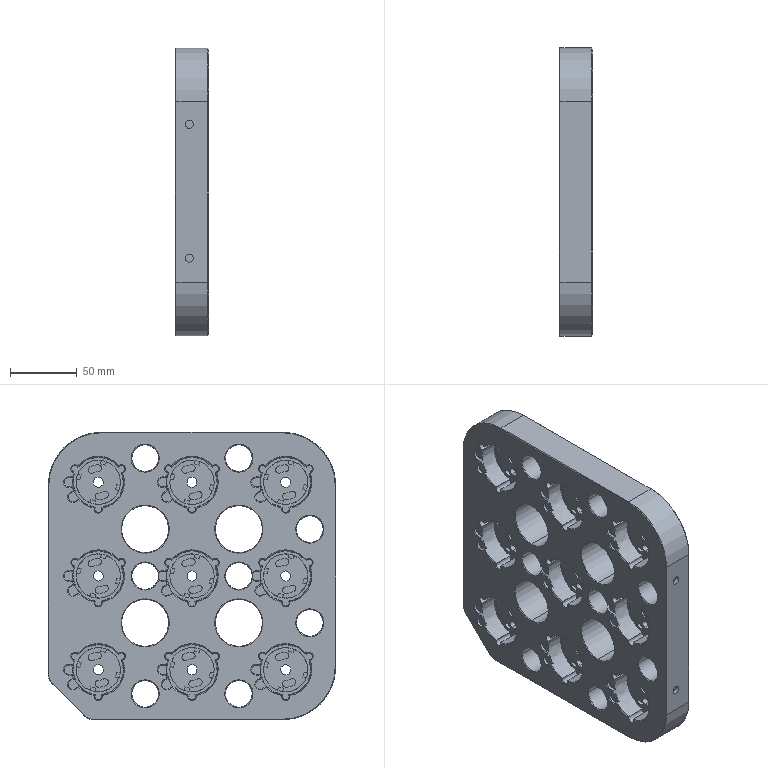Part | SolidWorks | features ICE 12, MoveCopyBody 7, LPattern 6, MoveFace 5, Chamfer 4, Cut 2, Fillet 2, Stock 2, Extrusion 1, HoleWzd 1 | 1 solid | 709 faces | box 25 x 215 x 215 mm | volume 792326 mm3 | plane 289 | cone 237 | cylinder 183 | commonest cylinder face diameters 5 x54 7 x20 7.5 x18 16.05 x18 20 x18 26.05 x18